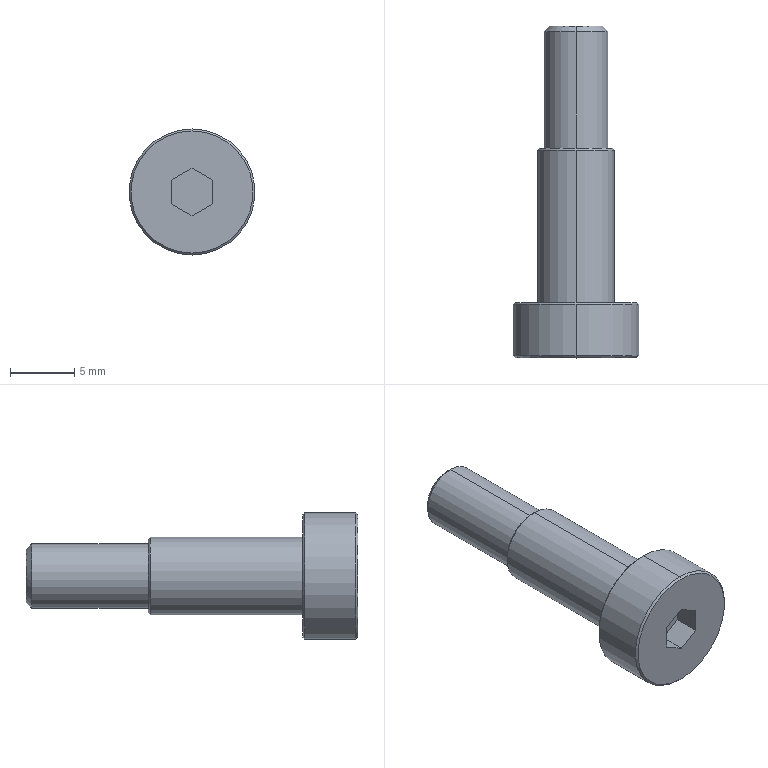Part | SolidWorks | features ICE 2, Chamfer 1, Extrusion 1, StudWizard 1 | 1 solid | 25 faces | box 9.8 x 25.8 x 9.8 mm | volume 830.154 mm3 | plane 11 | cone 8 | cylinder 6 | commonest cylinder face diameters 5 x2 6 x2 9.8 x2
STEP:
#1=CARTESIAN_POINT('',(0.,0.,-4.75));
#2=VERTEX_POINT('',#1);
#3=CARTESIAN_POINT('',(0.,0.,4.75));
#4=VERTEX_POINT('',#3);
#5=CARTESIAN_POINT('',(0.,0.,0.));
#6=DIRECTION('',(0.,-1.,0.));
#7=DIRECTION('',(0.,0.,1.));
#8=AXIS2_PLACEMENT_3D('',#5,#6,#7);
#9=CIRCLE('',#8,4.75);
#10=EDGE_CURVE('',#2,#4,#9,.T.);
#11=ORIENTED_EDGE('',*,*,#10,.F.);
#12=CARTESIAN_POINT('',(0.,0.15,-4.9));
#13=VERTEX_POINT('',#12);
#14=CARTESIAN_POINT('',(0.,0.15,-4.9));
#15=DIRECTION('',(0.,0.7071,-0.7071));
#16=VECTOR('',#15,1000.);
#17=LINE('',#14,#16);
#18=EDGE_CURVE('',#2,#13,#17,.T.);
#19=ORIENTED_EDGE('',*,*,#18,.T.);
#20=CARTESIAN_POINT('',(0.,0.15,4.9));
#21=VERTEX_POINT('',#20);
#22=CARTESIAN_POINT('',(0.,0.15,0.));
#23=DIRECTION('',(0.,1.,0.));
#24=DIRECTION('',(0.,0.,1.));
#25=AXIS2_PLACEMENT_3D('',#22,#23,#24);
#26=CIRCLE('',#25,4.9);
#27=EDGE_CURVE('',#21,#13,#26,.T.);
#28=ORIENTED_EDGE('',*,*,#27,.F.);
#29=CARTESIAN_POINT('',(0.,0.15,4.9));
#30=DIRECTION('',(0.,0.7071,0.7071));
#31=VECTOR('',#30,1000.);
#32=LINE('',#29,#31);
#33=EDGE_CURVE('',#4,#21,#32,.T.);
#34=ORIENTED_EDGE('',*,*,#33,.F.);
#35=EDGE_LOOP('',(#11,#19,#28,#34));
#36=FACE_OUTER_BOUND('',#35,.T.);
#37=CARTESIAN_POINT('',(0.,0.15,0.));
#38=DIRECTION('',(0.,1.,0.));
#39=DIRECTION('',(0.,0.,1.));
#40=AXIS2_PLACEMENT_3D('',#37,#38,#39);
#41=CONICAL_SURFACE('',#40,4.9,0.7854);
#42=ADVANCED_FACE('',(#36),#41,.T.);
#43=CARTESIAN_POINT('',(0.,4.3,4.75));
#44=VERTEX_POINT('',#43);
#45=CARTESIAN_POINT('',(0.,4.3,-4.75));
#46=VERTEX_POINT('',#45);
#47=CARTESIAN_POINT('',(0.,4.3,0.));
#48=DIRECTION('',(0.,1.,0.));
#49=DIRECTION('',(0.,0.,1.));
#50=AXIS2_PLACEMENT_3D('',#47,#48,#49);
#51=CIRCLE('',#50,4.75);
#52=EDGE_CURVE('',#44,#46,#51,.T.);
#53=ORIENTED_EDGE('',*,*,#52,.F.);
#54=CARTESIAN_POINT('',(0.,4.15,4.9));
#55=VERTEX_POINT('',#54);
#56=CARTESIAN_POINT('',(0.,4.3,4.75));
#57=DIRECTION('',(0.,-0.7071,0.7071));
#58=VECTOR('',#57,1000.);
#59=LINE('',#56,#58);
#60=EDGE_CURVE('',#44,#55,#59,.T.);
#61=ORIENTED_EDGE('',*,*,#60,.T.);
#62=CARTESIAN_POINT('',(0.,4.15,-4.9));
#63=VERTEX_POINT('',#62);
#64=CARTESIAN_POINT('',(0.,4.15,0.));
#65=DIRECTION('',(0.,-1.,0.));
#66=DIRECTION('',(0.,0.,1.));
#67=AXIS2_PLACEMENT_3D('',#64,#65,#66);
#68=CIRCLE('',#67,4.9);
#69=EDGE_CURVE('',#63,#55,#68,.T.);
#70=ORIENTED_EDGE('',*,*,#69,.F.);
#71=CARTESIAN_POINT('',(0.,4.3,-4.75));
#72=DIRECTION('',(0.,-0.7071,-0.7071));
#73=VECTOR('',#72,1000.);
#74=LINE('',#71,#73);
#75=EDGE_CURVE('',#46,#63,#74,.T.);
#76=ORIENTED_EDGE('',*,*,#75,.F.);
#77=EDGE_LOOP('',(#53,#61,#70,#76));
#78=FACE_OUTER_BOUND('',#77,.T.);
#79=CARTESIAN_POINT('',(0.,4.3,0.));
#80=DIRECTION('',(0.,-1.,0.));
#81=DIRECTION('',(0.,0.,-1.));
#82=AXIS2_PLACEMENT_3D('',#79,#80,#81);
#83=CONICAL_SURFACE('',#82,4.75,0.7854);
#84=ADVANCED_FACE('',(#78),#83,.T.);
#85=CARTESIAN_POINT('',(0.,16.3,2.85));
#86=VERTEX_POINT('',#85);
#87=CARTESIAN_POINT('',(0.,16.3,-2.85));
#88=VERTEX_POINT('',#87);
#89=CARTESIAN_POINT('',(0.,16.3,0.));
#90=DIRECTION('',(0.,1.,0.));
#91=DIRECTION('',(0.,0.,1.));
#92=AXIS2_PLACEMENT_3D('',#89,#90,#91);
#93=CIRCLE('',#92,2.85);
#94=EDGE_CURVE('',#86,#88,#93,.T.);
#95=ORIENTED_EDGE('',*,*,#94,.F.);
#96=CARTESIAN_POINT('',(0.,16.15,3.));
#97=VERTEX_POINT('',#96);
#98=CARTESIAN_POINT('',(0.,16.3,2.85));
#99=DIRECTION('',(0.,-0.7071,0.7071));
#100=VECTOR('',#99,1000.);
#101=LINE('',#98,#100);
#102=EDGE_CURVE('',#86,#97,#101,.T.);
#103=ORIENTED_EDGE('',*,*,#102,.T.);
#104=CARTESIAN_POINT('',(0.,16.15,-3.));
#105=VERTEX_POINT('',#104);
#106=CARTESIAN_POINT('',(0.,16.15,0.));
#107=DIRECTION('',(0.,-1.,0.));
#108=DIRECTION('',(0.,0.,1.));
#109=AXIS2_PLACEMENT_3D('',#106,#107,#108);
#110=CIRCLE('',#109,3.);
#111=EDGE_CURVE('',#105,#97,#110,.T.);
#112=ORIENTED_EDGE('',*,*,#111,.F.);
#113=CARTESIAN_POINT('',(0.,16.3,-2.85));
#114=DIRECTION('',(0.,-0.7071,-0.7071));
#115=VECTOR('',#114,1000.);
#116=LINE('',#113,#115);
#117=EDGE_CURVE('',#88,#105,#116,.T.);
#118=ORIENTED_EDGE('',*,*,#117,.F.);
#119=EDGE_LOOP('',(#95,#103,#112,#118));
#120=FACE_OUTER_BOUND('',#119,.T.);
#121=CARTESIAN_POINT('',(0.,16.3,0.));
#122=DIRECTION('',(0.,-1.,0.));
#123=DIRECTION('',(0.,0.,-1.));
#124=AXIS2_PLACEMENT_3D('',#121,#122,#123);
#125=CONICAL_SURFACE('',#124,2.85,0.7854);
#126=ADVANCED_FACE('',(#120),#125,.T.);
#127=CARTESIAN_POINT('',(0.,25.367,-2.5));
#128=VERTEX_POINT('',#127);
#129=CARTESIAN_POINT('',(0.,25.367,2.5));
#130=VERTEX_POINT('',#129);
#131=CARTESIAN_POINT('',(0.,25.367,0.));
#132=DIRECTION('',(0.,-1.,0.));
#133=DIRECTION('',(0.,0.,-1.));
#134=AXIS2_PLACEMENT_3D('',#131,#132,#133);
#135=CIRCLE('',#134,2.5);
#136=EDGE_CURVE('',#128,#130,#135,.T.);
#137=ORIENTED_EDGE('',*,*,#136,.T.);
#138=CARTESIAN_POINT('',(0.,16.3,2.5));
#139=VERTEX_POINT('',#138);
#140=CARTESIAN_POINT('',(0.,16.3,2.5));
#141=DIRECTION('',(0.,-1.,0.));
#142=VECTOR('',#141,1000.);
#143=LINE('',#140,#142);
#144=EDGE_CURVE('',#130,#139,#143,.T.);
#145=ORIENTED_EDGE('',*,*,#144,.T.);
#146=CARTESIAN_POINT('',(0.,16.3,-2.5));
#147=VERTEX_POINT('',#146);
#148=CARTESIAN_POINT('',(0.,16.3,0.));
#149=DIRECTION('',(0.,-1.,0.));
#150=DIRECTION('',(0.,0.,-1.));
#151=AXIS2_PLACEMENT_3D('',#148,#149,#150);
#152=CIRCLE('',#151,2.5);
#153=EDGE_CURVE('',#147,#139,#152,.T.);
#154=ORIENTED_EDGE('',*,*,#153,.F.);
#155=CARTESIAN_POINT('',(0.,16.3,-2.5));
#156=DIRECTION('',(0.,-1.,0.));
#157=VECTOR('',#156,1000.);
#158=LINE('',#155,#157);
#159=EDGE_CURVE('',#128,#147,#158,.T.);
#160=ORIENTED_EDGE('',*,*,#159,.F.);
#161=EDGE_LOOP('',(#137,#145,#154,#160));
#162=FACE_OUTER_BOUND('',#161,.T.);
#163=CARTESIAN_POINT('',(0.,16.3,0.));
#164=DIRECTION('',(0.,-1.,0.));
#165=DIRECTION('',(0.,0.,-1.));
#166=AXIS2_PLACEMENT_3D('',#163,#164,#165);
#167=CYLINDRICAL_SURFACE('',#166,2.5);
#168=ADVANCED_FACE('',(#162),#167,.T.);
#169=CARTESIAN_POINT('',(0.,25.8,-2.067));
#170=VERTEX_POINT('',#169);
#171=CARTESIAN_POINT('',(0.,25.8,2.067));
#172=VERTEX_POINT('',#171);
#173=CARTESIAN_POINT('',(0.,25.8,0.));
#174=DIRECTION('',(0.,-1.,0.));
#175=DIRECTION('',(0.,0.,-1.));
#176=AXIS2_PLACEMENT_3D('',#173,#174,#175);
#177=CIRCLE('',#176,2.067);
#178=EDGE_CURVE('',#170,#172,#177,.T.);
#179=ORIENTED_EDGE('',*,*,#178,.T.);
#180=CARTESIAN_POINT('',(0.,25.367,2.5));
#181=DIRECTION('',(0.,-0.7071,0.7071));
#182=VECTOR('',#181,1000.);
#183=LINE('',#180,#182);
#184=EDGE_CURVE('',#172,#130,#183,.T.);
#185=ORIENTED_EDGE('',*,*,#184,.T.);
#186=ORIENTED_EDGE('',*,*,#136,.F.);
#187=CARTESIAN_POINT('',(0.,25.367,-2.5));
#188=DIRECTION('',(0.,-0.7071,-0.7071));
#189=VECTOR('',#188,1000.);
#190=LINE('',#187,#189);
#191=EDGE_CURVE('',#170,#128,#190,.T.);
#192=ORIENTED_EDGE('',*,*,#191,.F.);
#193=EDGE_LOOP('',(#179,#185,#186,#192));
#194=FACE_OUTER_BOUND('',#193,.T.);
#195=CARTESIAN_POINT('',(0.,25.367,0.));
#196=DIRECTION('',(0.,-1.,0.));
#197=DIRECTION('',(0.,0.,-1.));
#198=AXIS2_PLACEMENT_3D('',#195,#196,#197);
#199=CONICAL_SURFACE('',#198,2.5,0.7854);
#200=ADVANCED_FACE('',(#194),#199,.T.);
#201=ORIENTED_EDGE('',*,*,#111,.T.);
#202=CARTESIAN_POINT('',(0.,4.3,3.));
#203=VERTEX_POINT('',#202);
#204=CARTESIAN_POINT('',(0.,16.3,3.));
#205=DIRECTION('',(0.,-1.,0.));
#206=VECTOR('',#205,1000.);
#207=LINE('',#204,#206);
#208=EDGE_CURVE('',#97,#203,#207,.T.);
#209=ORIENTED_EDGE('',*,*,#208,.T.);
#210=CARTESIAN_POINT('',(0.,4.3,-3.));
#211=VERTEX_POINT('',#210);
#212=CARTESIAN_POINT('',(0.,4.3,0.));
#213=DIRECTION('',(0.,1.,0.));
#214=DIRECTION('',(0.,0.,1.));
#215=AXIS2_PLACEMENT_3D('',#212,#213,#214);
#216=CIRCLE('',#215,3.);
#217=EDGE_CURVE('',#203,#211,#216,.T.);
#218=ORIENTED_EDGE('',*,*,#217,.T.);
#219=CARTESIAN_POINT('',(0.,16.3,-3.));
#220=DIRECTION('',(0.,-1.,0.));
#221=VECTOR('',#220,1000.);
#222=LINE('',#219,#221);
#223=EDGE_CURVE('',#105,#211,#222,.T.);
#224=ORIENTED_EDGE('',*,*,#223,.F.);
#225=EDGE_LOOP('',(#201,#209,#218,#224));
#226=FACE_OUTER_BOUND('',#225,.T.);
#227=CARTESIAN_POINT('',(0.,16.3,0.));
#228=DIRECTION('',(0.,-1.,0.));
#229=DIRECTION('',(0.,0.,-1.));
#230=AXIS2_PLACEMENT_3D('',#227,#228,#229);
#231=CYLINDRICAL_SURFACE('',#230,3.);
#232=ADVANCED_FACE('',(#226),#231,.T.);
#233=ORIENTED_EDGE('',*,*,#69,.T.);
#234=CARTESIAN_POINT('',(0.,4.3,4.9));
#235=DIRECTION('',(0.,-1.,0.));
#236=VECTOR('',#235,1000.);
#237=LINE('',#234,#236);
#238=EDGE_CURVE('',#55,#21,#237,.T.);
#239=ORIENTED_EDGE('',*,*,#238,.T.);
#240=ORIENTED_EDGE('',*,*,#27,.T.);
#241=CARTESIAN_POINT('',(0.,4.3,-4.9));
#242=DIRECTION('',(0.,-1.,0.));
#243=VECTOR('',#242,1000.);
#244=LINE('',#241,#243);
#245=EDGE_CURVE('',#63,#13,#244,.T.);
#246=ORIENTED_EDGE('',*,*,#245,.F.);
#247=EDGE_LOOP('',(#233,#239,#240,#246));
#248=FACE_OUTER_BOUND('',#247,.T.);
#249=CARTESIAN_POINT('',(0.,4.3,0.));
#250=DIRECTION('',(0.,-1.,0.));
#251=DIRECTION('',(0.,0.,-1.));
#252=AXIS2_PLACEMENT_3D('',#249,#250,#251);
#253=CYLINDRICAL_SURFACE('',#252,4.9);
#254=ADVANCED_FACE('',(#248),#253,.T.);
#255=ORIENTED_EDGE('',*,*,#238,.F.);
#256=CARTESIAN_POINT('',(0.,4.15,0.));
#257=DIRECTION('',(0.,-1.,0.));
#258=DIRECTION('',(0.,0.,1.));
#259=AXIS2_PLACEMENT_3D('',#256,#257,#258);
#260=CIRCLE('',#259,4.9);
#261=EDGE_CURVE('',#55,#63,#260,.T.);
#262=ORIENTED_EDGE('',*,*,#261,.T.);
#263=ORIENTED_EDGE('',*,*,#245,.T.);
#264=CARTESIAN_POINT('',(0.,0.15,0.));
#265=DIRECTION('',(0.,1.,0.));
#266=DIRECTION('',(0.,0.,1.));
#267=AXIS2_PLACEMENT_3D('',#264,#265,#266);
#268=CIRCLE('',#267,4.9);
#269=EDGE_CURVE('',#13,#21,#268,.T.);
#270=ORIENTED_EDGE('',*,*,#269,.T.);
#271=EDGE_LOOP('',(#255,#262,#263,#270));
#272=FACE_OUTER_BOUND('',#271,.T.);
#273=CARTESIAN_POINT('',(0.,4.3,0.));
#274=DIRECTION('',(0.,-1.,0.));
#275=DIRECTION('',(0.,0.,-1.));
#276=AXIS2_PLACEMENT_3D('',#273,#274,#275);
#277=CYLINDRICAL_SURFACE('',#276,4.9);
#278=ADVANCED_FACE('',(#272),#277,.T.);
#279=CARTESIAN_POINT('',(0.,4.3,0.));
#280=DIRECTION('',(0.,1.,0.));
#281=DIRECTION('',(0.,0.,1.));
#282=AXIS2_PLACEMENT_3D('',#279,#280,#281);
#283=CIRCLE('',#282,4.75);
#284=EDGE_CURVE('',#46,#44,#283,.T.);
#285=ORIENTED_EDGE('',*,*,#284,.T.);
#286=ORIENTED_EDGE('',*,*,#52,.T.);
#287=EDGE_LOOP('',(#285,#286));
#288=FACE_OUTER_BOUND('',#287,.T.);
#289=CARTESIAN_POINT('',(0.,4.3,0.));
#290=DIRECTION('',(0.,1.,0.));
#291=DIRECTION('',(0.,0.,1.));
#292=AXIS2_PLACEMENT_3D('',#289,#290,#291);
#293=CIRCLE('',#292,3.);
#294=EDGE_CURVE('',#211,#203,#293,.T.);
#295=ORIENTED_EDGE('',*,*,#294,.F.);
#296=ORIENTED_EDGE('',*,*,#217,.F.);
#297=EDGE_LOOP('',(#295,#296));
#298=FACE_BOUND('',#297,.T.);
#299=CARTESIAN_POINT('',(0.,4.3,0.));
#300=DIRECTION('',(0.,1.,0.));
#301=DIRECTION('',(0.,0.,1.));
#302=AXIS2_PLACEMENT_3D('',#299,#300,#301);
#303=PLANE('',#302);
#304=ADVANCED_FACE('',(#288,#298),#303,.T.);
#305=CARTESIAN_POINT('',(0.,0.,0.));
#306=DIRECTION('',(0.,-1.,0.));
#307=DIRECTION('',(0.,0.,1.));
#308=AXIS2_PLACEMENT_3D('',#305,#306,#307);
#309=CIRCLE('',#308,4.75);
#310=EDGE_CURVE('',#4,#2,#309,.T.);
#311=ORIENTED_EDGE('',*,*,#310,.T.);
#312=ORIENTED_EDGE('',*,*,#10,.T.);
#313=EDGE_LOOP('',(#311,#312));
#314=FACE_OUTER_BOUND('',#313,.T.);
#315=CARTESIAN_POINT('',(0.,0.,1.848));
#316=VERTEX_POINT('',#315);
#317=CARTESIAN_POINT('',(-1.6,0.,0.9238));
#318=VERTEX_POINT('',#317);
#319=CARTESIAN_POINT('',(0.,0.,1.848));
#320=DIRECTION('',(-0.866,0.,-0.5));
#321=VECTOR('',#320,1000.);
#322=LINE('',#319,#321);
#323=EDGE_CURVE('',#316,#318,#322,.T.);
#324=ORIENTED_EDGE('',*,*,#323,.F.);
#325=CARTESIAN_POINT('',(1.6,0.,0.9238));
#326=VERTEX_POINT('',#325);
#327=CARTESIAN_POINT('',(1.6,0.,0.9238));
#328=DIRECTION('',(-0.866,0.,0.5));
#329=VECTOR('',#328,1000.);
#330=LINE('',#327,#329);
#331=EDGE_CURVE('',#326,#316,#330,.T.);
#332=ORIENTED_EDGE('',*,*,#331,.F.);
#333=CARTESIAN_POINT('',(1.6,0.,-0.9238));
#334=VERTEX_POINT('',#333);
#335=CARTESIAN_POINT('',(1.6,0.,-0.9238));
#336=DIRECTION('',(0.,0.,1.));
#337=VECTOR('',#336,1000.);
#338=LINE('',#335,#337);
#339=EDGE_CURVE('',#334,#326,#338,.T.);
#340=ORIENTED_EDGE('',*,*,#339,.F.);
#341=CARTESIAN_POINT('',(0.,0.,-1.848));
#342=VERTEX_POINT('',#341);
#343=CARTESIAN_POINT('',(0.,0.,-1.848));
#344=DIRECTION('',(0.866,0.,0.5));
#345=VECTOR('',#344,1000.);
#346=LINE('',#343,#345);
#347=EDGE_CURVE('',#342,#334,#346,.T.);
#348=ORIENTED_EDGE('',*,*,#347,.F.);
#349=CARTESIAN_POINT('',(-1.6,0.,-0.9238));
#350=VERTEX_POINT('',#349);
#351=CARTESIAN_POINT('',(-1.6,0.,-0.9238));
#352=DIRECTION('',(0.866,0.,-0.5));
#353=VECTOR('',#352,1000.);
#354=LINE('',#351,#353);
#355=EDGE_CURVE('',#350,#342,#354,.T.);
#356=ORIENTED_EDGE('',*,*,#355,.F.);
#357=CARTESIAN_POINT('',(-1.6,0.,0.9238));
#358=DIRECTION('',(0.,0.,-1.));
#359=VECTOR('',#358,1000.);
#360=LINE('',#357,#359);
#361=EDGE_CURVE('',#318,#350,#360,.T.);
#362=ORIENTED_EDGE('',*,*,#361,.F.);
#363=EDGE_LOOP('',(#324,#332,#340,#348,#356,#362));
#364=FACE_BOUND('',#363,.T.);
#365=CARTESIAN_POINT('',(0.,0.,0.));
#366=DIRECTION('',(0.,1.,0.));
#367=DIRECTION('',(0.,0.,1.));
#368=AXIS2_PLACEMENT_3D('',#365,#366,#367);
#369=PLANE('',#368);
#370=ADVANCED_FACE('',(#314,#364),#369,.F.);
#371=ORIENTED_EDGE('',*,*,#208,.F.);
#372=CARTESIAN_POINT('',(0.,16.15,0.));
#373=DIRECTION('',(0.,-1.,0.));
#374=DIRECTION('',(0.,0.,1.));
#375=AXIS2_PLACEMENT_3D('',#372,#373,#374);
#376=CIRCLE('',#375,3.);
#377=EDGE_CURVE('',#97,#105,#376,.T.);
#378=ORIENTED_EDGE('',*,*,#377,.T.);
#379=ORIENTED_EDGE('',*,*,#223,.T.);
#380=ORIENTED_EDGE('',*,*,#294,.T.);
#381=EDGE_LOOP('',(#371,#378,#379,#380));
#382=FACE_OUTER_BOUND('',#381,.T.);
#383=CARTESIAN_POINT('',(0.,16.3,0.));
#384=DIRECTION('',(0.,-1.,0.));
#385=DIRECTION('',(0.,0.,-1.));
#386=AXIS2_PLACEMENT_3D('',#383,#384,#385);
#387=CYLINDRICAL_SURFACE('',#386,3.);
#388=ADVANCED_FACE('',(#382),#387,.T.);
#389=CARTESIAN_POINT('',(0.,16.3,0.));
#390=DIRECTION('',(0.,1.,0.));
#391=DIRECTION('',(0.,0.,1.));
#392=AXIS2_PLACEMENT_3D('',#389,#390,#391);
#393=CIRCLE('',#392,2.85);
#394=EDGE_CURVE('',#88,#86,#393,.T.);
#395=ORIENTED_EDGE('',*,*,#394,.T.);
#396=ORIENTED_EDGE('',*,*,#94,.T.);
#397=EDGE_LOOP('',(#395,#396));
#398=FACE_OUTER_BOUND('',#397,.T.);
#399=ORIENTED_EDGE('',*,*,#153,.T.);
#400=CARTESIAN_POINT('',(0.,16.3,0.));
#401=DIRECTION('',(0.,-1.,0.));
#402=DIRECTION('',(0.,0.,-1.));
#403=AXIS2_PLACEMENT_3D('',#400,#401,#402);
#404=CIRCLE('',#403,2.5);
#405=EDGE_CURVE('',#139,#147,#404,.T.);
#406=ORIENTED_EDGE('',*,*,#405,.T.);
#407=EDGE_LOOP('',(#399,#406));
#408=FACE_BOUND('',#407,.T.);
#409=CARTESIAN_POINT('',(0.,16.3,0.));
#410=DIRECTION('',(0.,1.,0.));
#411=DIRECTION('',(0.,0.,1.));
#412=AXIS2_PLACEMENT_3D('',#409,#410,#411);
#413=PLANE('',#412);
#414=ADVANCED_FACE('',(#398,#408),#413,.T.);
#415=ORIENTED_EDGE('',*,*,#178,.F.);
#416=CARTESIAN_POINT('',(0.,25.8,0.));
#417=DIRECTION('',(0.,-1.,0.));
#418=DIRECTION('',(0.,0.,-1.));
#419=AXIS2_PLACEMENT_3D('',#416,#417,#418);
#420=CIRCLE('',#419,2.067);
#421=EDGE_CURVE('',#172,#170,#420,.T.);
#422=ORIENTED_EDGE('',*,*,#421,.F.);
#423=EDGE_LOOP('',(#415,#422));
#424=FACE_OUTER_BOUND('',#423,.T.);
#425=CARTESIAN_POINT('',(2.067,25.8,0.));
#426=DIRECTION('',(0.,1.,0.));
#427=DIRECTION('',(0.,0.,1.));
#428=AXIS2_PLACEMENT_3D('',#425,#426,#427);
#429=PLANE('',#428);
#430=ADVANCED_FACE('',(#424),#429,.T.);
#431=ORIENTED_EDGE('',*,*,#184,.F.);
#432=ORIENTED_EDGE('',*,*,#421,.T.);
#433=ORIENTED_EDGE('',*,*,#191,.T.);
#434=CARTESIAN_POINT('',(0.,25.367,0.));
#435=DIRECTION('',(0.,-1.,0.));
#436=DIRECTION('',(0.,0.,-1.));
#437=AXIS2_PLACEMENT_3D('',#434,#435,#436);
#438=CIRCLE('',#437,2.5);
#439=EDGE_CURVE('',#130,#128,#438,.T.);
#440=ORIENTED_EDGE('',*,*,#439,.F.);
#441=EDGE_LOOP('',(#431,#432,#433,#440));
#442=FACE_OUTER_BOUND('',#441,.T.);
#443=CARTESIAN_POINT('',(0.,25.367,0.));
#444=DIRECTION('',(0.,-1.,0.));
#445=DIRECTION('',(0.,0.,-1.));
#446=AXIS2_PLACEMENT_3D('',#443,#444,#445);
#447=CONICAL_SURFACE('',#446,2.5,0.7854);
#448=ADVANCED_FACE('',(#442),#447,.T.);
#449=ORIENTED_EDGE('',*,*,#144,.F.);
#450=ORIENTED_EDGE('',*,*,#439,.T.);
#451=ORIENTED_EDGE('',*,*,#159,.T.);
#452=ORIENTED_EDGE('',*,*,#405,.F.);
#453=EDGE_LOOP('',(#449,#450,#451,#452));
#454=FACE_OUTER_BOUND('',#453,.T.);
#455=CARTESIAN_POINT('',(0.,16.3,0.));
#456=DIRECTION('',(0.,-1.,0.));
#457=DIRECTION('',(0.,0.,-1.));
#458=AXIS2_PLACEMENT_3D('',#455,#456,#457);
#459=CYLINDRICAL_SURFACE('',#458,2.5);
#460=ADVANCED_FACE('',(#454),#459,.T.);
#461=ORIENTED_EDGE('',*,*,#331,.T.);
#462=CARTESIAN_POINT('',(0.,2.,1.848));
#463=VERTEX_POINT('',#462);
#464=CARTESIAN_POINT('',(0.,2.,1.848));
#465=DIRECTION('',(0.,-1.,0.));
#466=VECTOR('',#465,1000.);
#467=LINE('',#464,#466);
#468=EDGE_CURVE('',#463,#316,#467,.T.);
#469=ORIENTED_EDGE('',*,*,#468,.F.);
#470=CARTESIAN_POINT('',(1.6,2.,0.9238));
#471=VERTEX_POINT('',#470);
#472=CARTESIAN_POINT('',(1.6,2.,0.9238));
#473=DIRECTION('',(-0.866,0.,0.5));
#474=VECTOR('',#473,1000.);
#475=LINE('',#472,#474);
#476=EDGE_CURVE('',#471,#463,#475,.T.);
#477=ORIENTED_EDGE('',*,*,#476,.F.);
#478=CARTESIAN_POINT('',(1.6,2.,0.9238));
#479=DIRECTION('',(0.,-1.,0.));
#480=VECTOR('',#479,1000.);
#481=LINE('',#478,#480);
#482=EDGE_CURVE('',#471,#326,#481,.T.);
#483=ORIENTED_EDGE('',*,*,#482,.T.);
#484=EDGE_LOOP('',(#461,#469,#477,#483));
#485=FACE_OUTER_BOUND('',#484,.T.);
#486=CARTESIAN_POINT('',(1.6,2.,0.9238));
#487=DIRECTION('',(0.5,0.,0.866));
#488=DIRECTION('',(0.866,0.,-0.5));
#489=AXIS2_PLACEMENT_3D('',#486,#487,#488);
#490=PLANE('',#489);
#491=ADVANCED_FACE('',(#485),#490,.F.);
#492=ORIENTED_EDGE('',*,*,#339,.T.);
#493=ORIENTED_EDGE('',*,*,#482,.F.);
#494=CARTESIAN_POINT('',(1.6,2.,-0.9238));
#495=VERTEX_POINT('',#494);
#496=CARTESIAN_POINT('',(1.6,2.,-0.9238));
#497=DIRECTION('',(0.,0.,1.));
#498=VECTOR('',#497,1000.);
#499=LINE('',#496,#498);
#500=EDGE_CURVE('',#495,#471,#499,.T.);
#501=ORIENTED_EDGE('',*,*,#500,.F.);
#502=CARTESIAN_POINT('',(1.6,2.,-0.9238));
#503=DIRECTION('',(0.,-1.,0.));
#504=VECTOR('',#503,1000.);
#505=LINE('',#502,#504);
#506=EDGE_CURVE('',#495,#334,#505,.T.);
#507=ORIENTED_EDGE('',*,*,#506,.T.);
#508=EDGE_LOOP('',(#492,#493,#501,#507));
#509=FACE_OUTER_BOUND('',#508,.T.);
#510=CARTESIAN_POINT('',(1.6,2.,-0.9238));
#511=DIRECTION('',(1.,0.,0.));
#512=DIRECTION('',(0.,0.,-1.));
#513=AXIS2_PLACEMENT_3D('',#510,#511,#512);
#514=PLANE('',#513);
#515=ADVANCED_FACE('',(#509),#514,.F.);
#516=ORIENTED_EDGE('',*,*,#347,.T.);
#517=ORIENTED_EDGE('',*,*,#506,.F.);
#518=CARTESIAN_POINT('',(0.,2.,-1.848));
#519=VERTEX_POINT('',#518);
#520=CARTESIAN_POINT('',(0.,2.,-1.848));
#521=DIRECTION('',(0.866,0.,0.5));
#522=VECTOR('',#521,1000.);
#523=LINE('',#520,#522);
#524=EDGE_CURVE('',#519,#495,#523,.T.);
#525=ORIENTED_EDGE('',*,*,#524,.F.);
#526=CARTESIAN_POINT('',(0.,2.,-1.848));
#527=DIRECTION('',(0.,-1.,0.));
#528=VECTOR('',#527,1000.);
#529=LINE('',#526,#528);
#530=EDGE_CURVE('',#519,#342,#529,.T.);
#531=ORIENTED_EDGE('',*,*,#530,.T.);
#532=EDGE_LOOP('',(#516,#517,#525,#531));
#533=FACE_OUTER_BOUND('',#532,.T.);
#534=CARTESIAN_POINT('',(0.,2.,-1.848));
#535=DIRECTION('',(0.5,0.,-0.866));
#536=DIRECTION('',(-0.866,0.,-0.5));
#537=AXIS2_PLACEMENT_3D('',#534,#535,#536);
#538=PLANE('',#537);
#539=ADVANCED_FACE('',(#533),#538,.F.);
#540=ORIENTED_EDGE('',*,*,#355,.T.);
#541=ORIENTED_EDGE('',*,*,#530,.F.);
#542=CARTESIAN_POINT('',(-1.6,2.,-0.9238));
#543=VERTEX_POINT('',#542);
#544=CARTESIAN_POINT('',(-1.6,2.,-0.9238));
#545=DIRECTION('',(0.866,0.,-0.5));
#546=VECTOR('',#545,1000.);
#547=LINE('',#544,#546);
#548=EDGE_CURVE('',#543,#519,#547,.T.);
#549=ORIENTED_EDGE('',*,*,#548,.F.);
#550=CARTESIAN_POINT('',(-1.6,2.,-0.9238));
#551=DIRECTION('',(0.,-1.,0.));
#552=VECTOR('',#551,1000.);
#553=LINE('',#550,#552);
#554=EDGE_CURVE('',#543,#350,#553,.T.);
#555=ORIENTED_EDGE('',*,*,#554,.T.);
#556=EDGE_LOOP('',(#540,#541,#549,#555));
#557=FACE_OUTER_BOUND('',#556,.T.);
#558=CARTESIAN_POINT('',(-1.6,2.,-0.9238));
#559=DIRECTION('',(-0.5,0.,-0.866));
#560=DIRECTION('',(-0.866,0.,0.5));
#561=AXIS2_PLACEMENT_3D('',#558,#559,#560);
#562=PLANE('',#561);
#563=ADVANCED_FACE('',(#557),#562,.F.);
#564=ORIENTED_EDGE('',*,*,#361,.T.);
#565=ORIENTED_EDGE('',*,*,#554,.F.);
#566=CARTESIAN_POINT('',(-1.6,2.,0.9238));
#567=VERTEX_POINT('',#566);
#568=CARTESIAN_POINT('',(-1.6,2.,0.9238));
#569=DIRECTION('',(0.,0.,-1.));
#570=VECTOR('',#569,1000.);
#571=LINE('',#568,#570);
#572=EDGE_CURVE('',#567,#543,#571,.T.);
#573=ORIENTED_EDGE('',*,*,#572,.F.);
#574=CARTESIAN_POINT('',(-1.6,2.,0.9238));
#575=DIRECTION('',(0.,-1.,0.));
#576=VECTOR('',#575,1000.);
#577=LINE('',#574,#576);
#578=EDGE_CURVE('',#567,#318,#577,.T.);
#579=ORIENTED_EDGE('',*,*,#578,.T.);
#580=EDGE_LOOP('',(#564,#565,#573,#579));
#581=FACE_OUTER_BOUND('',#580,.T.);
#582=CARTESIAN_POINT('',(-1.6,2.,0.9238));
#583=DIRECTION('',(-1.,0.,0.));
#584=DIRECTION('',(0.,0.,1.));
#585=AXIS2_PLACEMENT_3D('',#582,#583,#584);
#586=PLANE('',#585);
#587=ADVANCED_FACE('',(#581),#586,.F.);
#588=ORIENTED_EDGE('',*,*,#323,.T.);
#589=ORIENTED_EDGE('',*,*,#578,.F.);
#590=CARTESIAN_POINT('',(0.,2.,1.848));
#591=DIRECTION('',(-0.866,0.,-0.5));
#592=VECTOR('',#591,1000.);
#593=LINE('',#590,#592);
#594=EDGE_CURVE('',#463,#567,#593,.T.);
#595=ORIENTED_EDGE('',*,*,#594,.F.);
#596=ORIENTED_EDGE('',*,*,#468,.T.);
#597=EDGE_LOOP('',(#588,#589,#595,#596));
#598=FACE_OUTER_BOUND('',#597,.T.);
#599=CARTESIAN_POINT('',(0.,2.,1.848));
#600=DIRECTION('',(-0.5,0.,0.866));
#601=DIRECTION('',(0.866,0.,0.5));
#602=AXIS2_PLACEMENT_3D('',#599,#600,#601);
#603=PLANE('',#602);
#604=ADVANCED_FACE('',(#598),#603,.F.);
#605=ORIENTED_EDGE('',*,*,#476,.T.);
#606=ORIENTED_EDGE('',*,*,#594,.T.);
#607=ORIENTED_EDGE('',*,*,#572,.T.);
#608=ORIENTED_EDGE('',*,*,#548,.T.);
#609=ORIENTED_EDGE('',*,*,#524,.T.);
#610=ORIENTED_EDGE('',*,*,#500,.T.);
#611=EDGE_LOOP('',(#605,#606,#607,#608,#609,#610));
#612=FACE_OUTER_BOUND('',#611,.T.);
#613=CARTESIAN_POINT('',(0.,2.,0.));
#614=DIRECTION('',(0.,-1.,0.));
#615=DIRECTION('',(0.,0.,-1.));
#616=AXIS2_PLACEMENT_3D('',#613,#614,#615);
#617=PLANE('',#616);
#618=ADVANCED_FACE('',(#612),#617,.T.);
#619=ORIENTED_EDGE('',*,*,#102,.F.);
#620=ORIENTED_EDGE('',*,*,#394,.F.);
#621=ORIENTED_EDGE('',*,*,#117,.T.);
#622=ORIENTED_EDGE('',*,*,#377,.F.);
#623=EDGE_LOOP('',(#619,#620,#621,#622));
#624=FACE_OUTER_BOUND('',#623,.T.);
#625=CARTESIAN_POINT('',(0.,16.3,0.));
#626=DIRECTION('',(0.,-1.,0.));
#627=DIRECTION('',(0.,0.,-1.));
#628=AXIS2_PLACEMENT_3D('',#625,#626,#627);
#629=CONICAL_SURFACE('',#628,2.85,0.7854);
#630=ADVANCED_FACE('',(#624),#629,.T.);
#631=ORIENTED_EDGE('',*,*,#60,.F.);
#632=ORIENTED_EDGE('',*,*,#284,.F.);
#633=ORIENTED_EDGE('',*,*,#75,.T.);
#634=ORIENTED_EDGE('',*,*,#261,.F.);
#635=EDGE_LOOP('',(#631,#632,#633,#634));
#636=FACE_OUTER_BOUND('',#635,.T.);
#637=CARTESIAN_POINT('',(0.,4.3,0.));
#638=DIRECTION('',(0.,-1.,0.));
#639=DIRECTION('',(0.,0.,-1.));
#640=AXIS2_PLACEMENT_3D('',#637,#638,#639);
#641=CONICAL_SURFACE('',#640,4.75,0.7854);
#642=ADVANCED_FACE('',(#636),#641,.T.);
#643=ORIENTED_EDGE('',*,*,#18,.F.);
#644=ORIENTED_EDGE('',*,*,#310,.F.);
#645=ORIENTED_EDGE('',*,*,#33,.T.);
#646=ORIENTED_EDGE('',*,*,#269,.F.);
#647=EDGE_LOOP('',(#643,#644,#645,#646));
#648=FACE_OUTER_BOUND('',#647,.T.);
#649=CARTESIAN_POINT('',(0.,0.15,0.));
#650=DIRECTION('',(0.,1.,0.));
#651=DIRECTION('',(0.,0.,1.));
#652=AXIS2_PLACEMENT_3D('',#649,#650,#651);
#653=CONICAL_SURFACE('',#652,4.9,0.7854);
#654=ADVANCED_FACE('',(#648),#653,.T.);
#655=CLOSED_SHELL('',(#42,#84,#126,#168,#200,#232,#254,#278,#304,#370,#388,#414,#430,#448,#460,#491,#515,#539,#563,#587,#604,#618,#630,#642,#654));
#656=MANIFOLD_SOLID_BREP('',#655);
#657=CARTESIAN_POINT('',(0.,0.,0.));
#658=DIRECTION('',(0.,0.,1.));
#659=DIRECTION('',(1.,0.,0.));
#660=AXIS2_PLACEMENT_3D('',#657,#658,#659);
#661=(LENGTH_UNIT()NAMED_UNIT(*)SI_UNIT(.MILLI.,.METRE.));
#662=UNCERTAINTY_MEASURE_WITH_UNIT(LENGTH_MEASURE(0.00001),#661,'','');
#663=(NAMED_UNIT(*)PLANE_ANGLE_UNIT()SI_UNIT($,.RADIAN.));
#664=(NAMED_UNIT(*)SI_UNIT($,.STERADIAN.)SOLID_ANGLE_UNIT());
#665=(GEOMETRIC_REPRESENTATION_CONTEXT(3)GLOBAL_UNCERTAINTY_ASSIGNED_CONTEXT((#662))GLOBAL_UNIT_ASSIGNED_CONTEXT((#661,#663,#664))REPRESENTATION_CONTEXT('',''));
#666=ADVANCED_BREP_SHAPE_REPRESENTATION('',(#656,#660),#665);